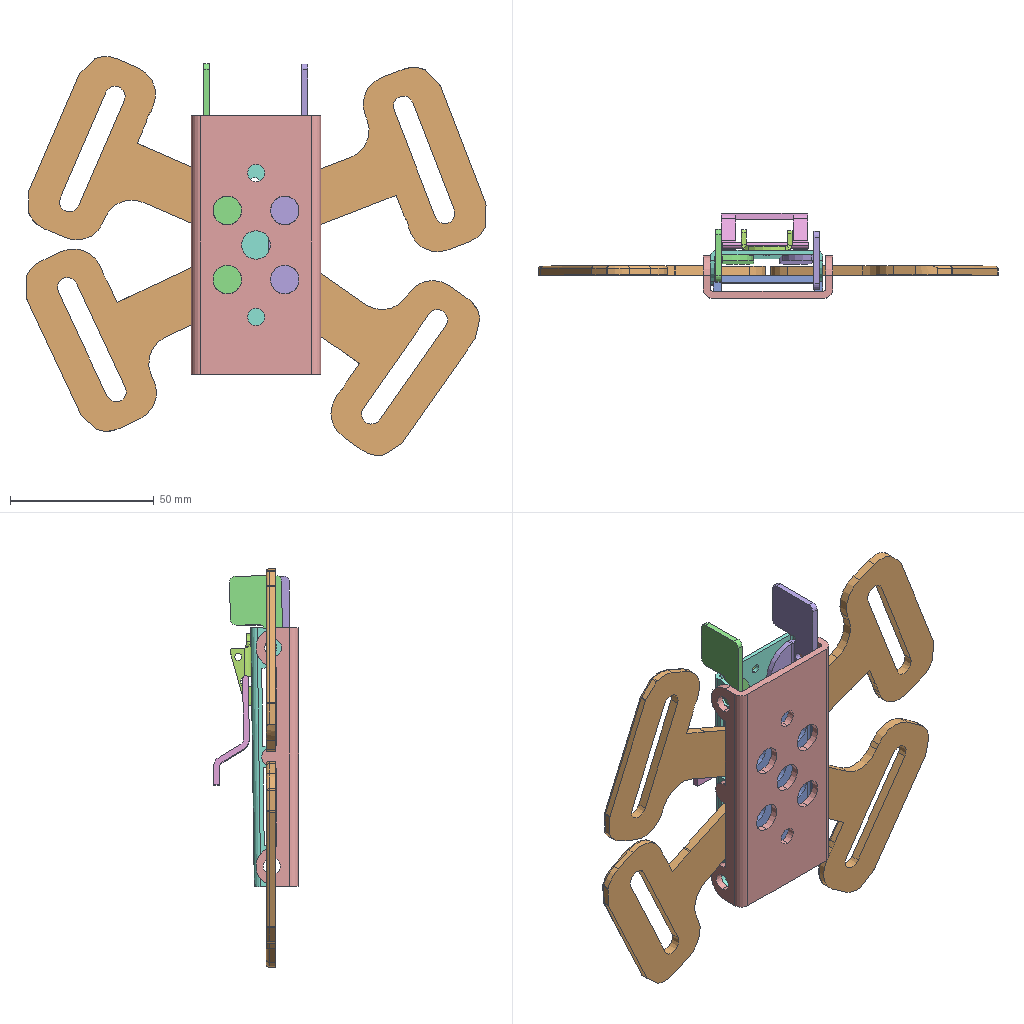Assembly | SolidWorks | 8 different items | 11 placed | box 160 x 30 x 138 mm
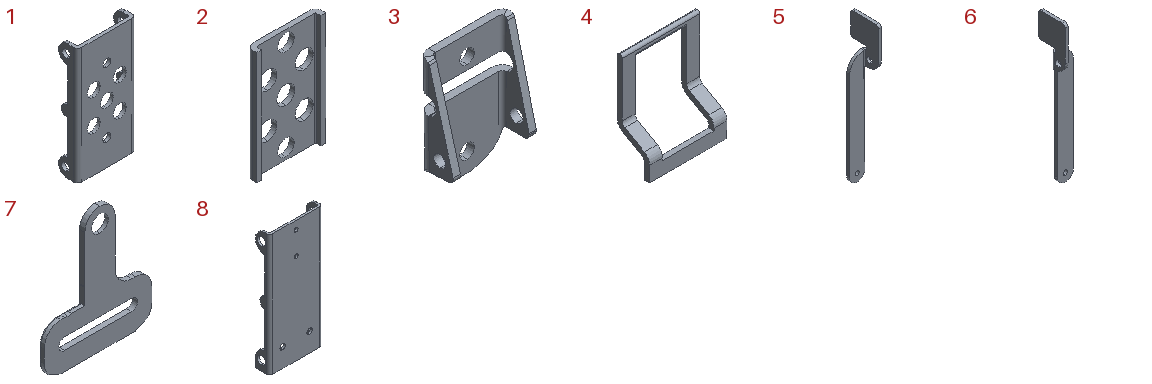Parts list (item | quantity | size | volume | features):
1 | x1 | 45 x 14.855 x 90 mm | 11672 mm3 | features HoleWzd 4, Fillet 2, ICE 2, Extrusion 1
2 | x1 | 37.996 x 5.595 x 62 mm | 5626 mm3 | features Fillet 2, HoleWzd 2, Extrusion 1, ICE 1
3 | x1 | 17.668 x 7.243 x 25.011 mm | 631.719 mm3 | features Fillet 3, HoleWzd 3, BaseBody 1
4 | x1 | 30 x 12.599 x 37.526 mm | 1159 mm3 | features ICE 9, Draft 2, Fillet 2, Extrusion 1
5 | x1 | 13 x 20.187 x 99.625 mm | 2561 mm3 | features Fillet 5, HoleWzd 2, BaseBody 1, ICE 1
6 | x1 | 13.227 x 18.048 x 99.5 mm | 2443 mm3 | features Fillet 4, HoleWzd 2, BaseBody 1, Draft 1, ICE 1
7 | x4 | 64.199 x 3.15 x 75 mm | 6691 mm3 | features Fillet 5, ICE 3, Chamfer 1, Extrusion 1, HoleWzd 1
8 | x1 | 39 x 10.638 x 90 mm | 6007 mm3 | features HoleWzd 4, Fillet 2, ICE 2, Extrusion 1
Mates (type | each side: item.copy, entity, surface, feature):
Coincident | 1.1 face plane Boss-Extrude2 | 2.1 face plane Boss-Extrude1
Concentric | 1.1 face cylinder Ø10.0 (10) Diameter Hole1 | 2.1 face cylinder Ø10.0 (10) Diameter Hole1
Concentric | 1.1 face cylinder Ø6.0 (6) Diameter Hole3 | 2.1 face cylinder Ø9.0 (9) Diameter Hole1
Concentric | 1.1 face cylinder Ø6.0 (6) Diameter Hole2 | 8.1 face cylinder Ø6.0 (6) Diameter Hole1
Coincident | 1.1 face plane Boss-Extrude1 | 8.1 face plane Boss-Extrude3
Concentric | 3.1 face cylinder Ø3.0 (3) Diameter Hole1 | 8.1 face cylinder Ø3.0 (3) Diameter Hole1 | 2 times
Coincident | 3.1 face plane Input 3 | 8.1 face plane Boss-Extrude1
Concentric | 8.1 face cylinder Ø4.0 (4) Diameter Hole1 | 6.1 face cylinder Ø3.0 (3) Diameter Hole1
Coincident | 8.1 face plane Boss-Extrude2 | 6.1 face plane Input 3
Concentric | 8.1 face cylinder Ø4.0 (4) Diameter Hole1 | 5.1 face cylinder M2.5 Clearance Hole1
Coincident | 8.1 face plane Boss-Extrude2 | 5.1 face plane Input 3
Concentric | 3.1 face cylinder Input 3 | 4.1 face cylinder Boss-Extrude1
Concentric | 1.1 face cylinder Ø10.0 (10) Diameter Hole1 | 7.1 face cylinder Ø10.0 (10) Diameter Hole1
Coincident | 2.1 face plane Boss-Extrude1 | 7.1 face plane Boss-Extrude1
Concentric | 2.1 face cylinder Ø10.0 (10) Diameter Hole1 | 7.2 face cylinder Ø10.0 (10) Diameter Hole1
Coincident | 2.1 face plane Boss-Extrude1 | 7.2 face plane Boss-Extrude1
Concentric | 2.1 face cylinder Ø10.0 (10) Diameter Hole1 | 7.3 face cylinder Ø10.0 (10) Diameter Hole1
Coincident | 2.1 face plane Boss-Extrude1 | 7.3 face plane Boss-Extrude1
Parallel | 8.1 face plane Boss-Extrude1 | 5.1 face plane Input 3
Parallel | 8.1 face plane Boss-Extrude3 | 6.1 face plane Input 3
Parallel | 4.1 face plane Boss-Extrude1 | 8.1 face plane Boss-Extrude1
DistanceDim | 4.1 face plane Boss-Extrude2 | 3.1 face plane Input 3
Concentric | 2.1 face cylinder Ø10.0 (10) Diameter Hole1 | 7.4 face cylinder Ø10.0 (10) Diameter Hole1
Coincident | 2.1 face plane Boss-Extrude1 | 7.4 face plane Boss-Extrude1